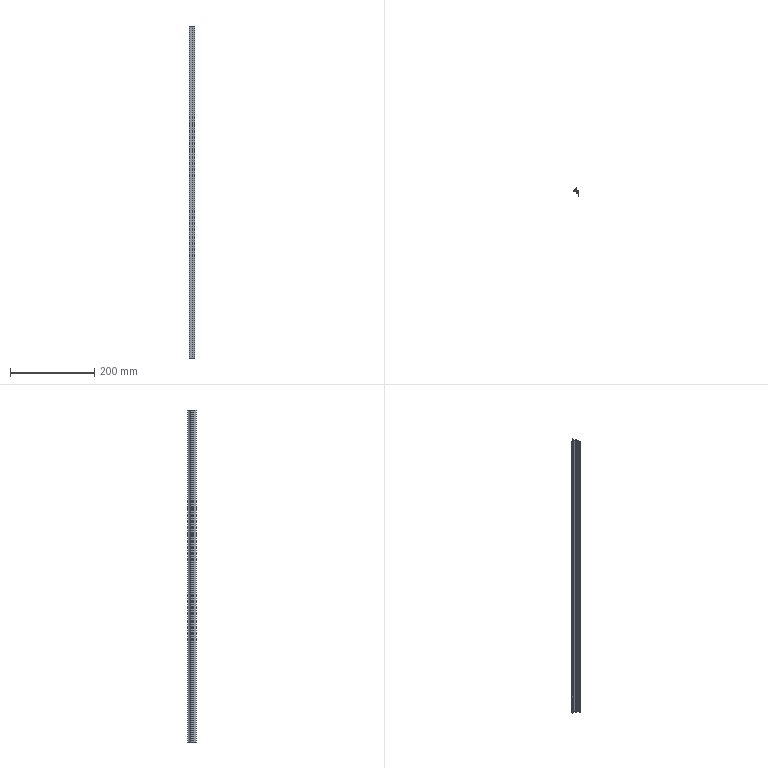Part | SolidWorks | features BaseBody 1, ICE 1, MoveFace 1 | 1 solid | 27 faces | box 14 x 20.3 x 786 mm | volume 40020 mm3 | plane 20 | cylinder 7 | commonest cylinder face diameters 0.387 x2 0.8 x2 0.4 x1 20 x1 22 x1
STEP:
#1=CARTESIAN_POINT('',(-5.304,-0.625,200.));
#2=VERTEX_POINT('',#1);
#3=CARTESIAN_POINT('',(-5.449,-0.8125,200.));
#4=VERTEX_POINT('',#3);
#5=CARTESIAN_POINT('',(-5.255,-0.8125,200.));
#6=DIRECTION('',(0.,0.,1.));
#7=DIRECTION('',(-1.,0.,0.));
#8=AXIS2_PLACEMENT_3D('',#5,#6,#7);
#9=CIRCLE('',#8,0.1937);
#10=EDGE_CURVE('',#2,#4,#9,.T.);
#11=ORIENTED_EDGE('',*,*,#10,.T.);
#12=CARTESIAN_POINT('',(-5.449,-0.8125,-586.));
#13=VERTEX_POINT('',#12);
#14=CARTESIAN_POINT('',(-5.449,-0.8125,230.));
#15=DIRECTION('',(0.,0.,-1.));
#16=VECTOR('',#15,1000.);
#17=LINE('',#14,#16);
#18=EDGE_CURVE('',#4,#13,#17,.T.);
#19=ORIENTED_EDGE('',*,*,#18,.T.);
#20=CARTESIAN_POINT('',(-5.304,-0.625,-586.));
#21=VERTEX_POINT('',#20);
#22=CARTESIAN_POINT('',(-5.255,-0.8125,-586.));
#23=DIRECTION('',(0.,0.,-1.));
#24=DIRECTION('',(1.,0.,0.));
#25=AXIS2_PLACEMENT_3D('',#22,#23,#24);
#26=CIRCLE('',#25,0.1937);
#27=EDGE_CURVE('',#13,#21,#26,.T.);
#28=ORIENTED_EDGE('',*,*,#27,.T.);
#29=CARTESIAN_POINT('',(-5.304,-0.625,230.));
#30=DIRECTION('',(0.,0.,-1.));
#31=VECTOR('',#30,1000.);
#32=LINE('',#29,#31);
#33=EDGE_CURVE('',#2,#21,#32,.T.);
#34=ORIENTED_EDGE('',*,*,#33,.F.);
#35=EDGE_LOOP('',(#11,#19,#28,#34));
#36=FACE_OUTER_BOUND('',#35,.T.);
#37=CARTESIAN_POINT('',(-5.255,-0.8125,230.));
#38=DIRECTION('',(0.,0.,-1.));
#39=DIRECTION('',(-1.,0.,0.));
#40=AXIS2_PLACEMENT_3D('',#37,#38,#39);
#41=CYLINDRICAL_SURFACE('',#40,0.1937);
#42=ADVANCED_FACE('',(#36),#41,.F.);
#43=CARTESIAN_POINT('',(5.,-1.,-586.));
#44=VERTEX_POINT('',#43);
#45=CARTESIAN_POINT('',(5.,-14.3,-586.));
#46=VERTEX_POINT('',#45);
#47=CARTESIAN_POINT('',(5.,29.623,-586.));
#48=DIRECTION('',(0.,-1.,0.));
#49=VECTOR('',#48,1000.);
#50=LINE('',#47,#49);
#51=EDGE_CURVE('',#44,#46,#50,.T.);
#52=ORIENTED_EDGE('',*,*,#51,.F.);
#53=CARTESIAN_POINT('',(5.,-1.,200.));
#54=VERTEX_POINT('',#53);
#55=CARTESIAN_POINT('',(5.,-1.,230.));
#56=DIRECTION('',(0.,0.,-1.));
#57=VECTOR('',#56,1000.);
#58=LINE('',#55,#57);
#59=EDGE_CURVE('',#54,#44,#58,.T.);
#60=ORIENTED_EDGE('',*,*,#59,.F.);
#61=CARTESIAN_POINT('',(5.,-14.3,200.));
#62=VERTEX_POINT('',#61);
#63=CARTESIAN_POINT('',(5.,-14.3,200.));
#64=DIRECTION('',(0.,1.,0.));
#65=VECTOR('',#64,1000.);
#66=LINE('',#63,#65);
#67=EDGE_CURVE('',#62,#54,#66,.T.);
#68=ORIENTED_EDGE('',*,*,#67,.F.);
#69=CARTESIAN_POINT('',(5.,-14.3,230.));
#70=DIRECTION('',(0.,0.,1.));
#71=VECTOR('',#70,1000.);
#72=LINE('',#69,#71);
#73=EDGE_CURVE('',#46,#62,#72,.T.);
#74=ORIENTED_EDGE('',*,*,#73,.F.);
#75=EDGE_LOOP('',(#52,#60,#68,#74));
#76=FACE_OUTER_BOUND('',#75,.T.);
#77=CARTESIAN_POINT('',(5.,-14.3,230.));
#78=DIRECTION('',(-1.,0.,0.));
#79=DIRECTION('',(0.,0.,1.));
#80=AXIS2_PLACEMENT_3D('',#77,#78,#79);
#81=PLANE('',#80);
#82=ADVANCED_FACE('',(#76),#81,.F.);
#83=CARTESIAN_POINT('',(-9.,-2.,-586.));
#84=VERTEX_POINT('',#83);
#85=CARTESIAN_POINT('',(-9.,-2.,200.));
#86=VERTEX_POINT('',#85);
#87=CARTESIAN_POINT('',(-9.,-2.,230.));
#88=DIRECTION('',(0.,0.,1.));
#89=VECTOR('',#88,1000.);
#90=LINE('',#87,#89);
#91=EDGE_CURVE('',#84,#86,#90,.T.);
#92=ORIENTED_EDGE('',*,*,#91,.F.);
#93=CARTESIAN_POINT('',(0.9,-2.,-586.));
#94=VERTEX_POINT('',#93);
#95=CARTESIAN_POINT('',(5.,-2.,-586.));
#96=DIRECTION('',(-1.,0.,0.));
#97=VECTOR('',#96,1000.);
#98=LINE('',#95,#97);
#99=EDGE_CURVE('',#94,#84,#98,.T.);
#100=ORIENTED_EDGE('',*,*,#99,.F.);
#101=CARTESIAN_POINT('',(0.9,-2.,200.));
#102=VERTEX_POINT('',#101);
#103=CARTESIAN_POINT('',(0.9,-2.,230.));
#104=DIRECTION('',(0.,0.,-1.));
#105=VECTOR('',#104,1000.);
#106=LINE('',#103,#105);
#107=EDGE_CURVE('',#102,#94,#106,.T.);
#108=ORIENTED_EDGE('',*,*,#107,.F.);
#109=CARTESIAN_POINT('',(5.,-2.,200.));
#110=DIRECTION('',(1.,0.,0.));
#111=VECTOR('',#110,1000.);
#112=LINE('',#109,#111);
#113=EDGE_CURVE('',#86,#102,#112,.T.);
#114=ORIENTED_EDGE('',*,*,#113,.F.);
#115=EDGE_LOOP('',(#92,#100,#108,#114));
#116=FACE_OUTER_BOUND('',#115,.T.);
#117=CARTESIAN_POINT('',(-9.,-2.,230.));
#118=DIRECTION('',(0.,1.,0.));
#119=DIRECTION('',(0.,0.,1.));
#120=AXIS2_PLACEMENT_3D('',#117,#118,#119);
#121=PLANE('',#120);
#122=ADVANCED_FACE('',(#116),#121,.F.);
#123=CARTESIAN_POINT('',(4.,-6.,200.));
#124=VERTEX_POINT('',#123);
#125=CARTESIAN_POINT('',(4.,-3.,200.));
#126=VERTEX_POINT('',#125);
#127=CARTESIAN_POINT('',(4.,29.623,200.));
#128=DIRECTION('',(0.,1.,0.));
#129=VECTOR('',#128,1000.);
#130=LINE('',#127,#129);
#131=EDGE_CURVE('',#124,#126,#130,.T.);
#132=ORIENTED_EDGE('',*,*,#131,.F.);
#133=CARTESIAN_POINT('',(1.,-6.,200.));
#134=VERTEX_POINT('',#133);
#135=CARTESIAN_POINT('',(5.,-6.,200.));
#136=DIRECTION('',(1.,0.,0.));
#137=VECTOR('',#136,1000.);
#138=LINE('',#135,#137);
#139=EDGE_CURVE('',#134,#124,#138,.T.);
#140=ORIENTED_EDGE('',*,*,#139,.F.);
#141=CARTESIAN_POINT('',(1.,-6.7,200.));
#142=VERTEX_POINT('',#141);
#143=CARTESIAN_POINT('',(1.,-6.,200.));
#144=DIRECTION('',(0.,-1.,0.));
#145=VECTOR('',#144,1000.);
#146=LINE('',#143,#145);
#147=EDGE_CURVE('',#134,#142,#146,.T.);
#148=ORIENTED_EDGE('',*,*,#147,.T.);
#149=CARTESIAN_POINT('',(-1.7,-6.7,200.));
#150=VERTEX_POINT('',#149);
#151=CARTESIAN_POINT('',(5.,-6.7,200.));
#152=DIRECTION('',(1.,0.,0.));
#153=VECTOR('',#152,1000.);
#154=LINE('',#151,#153);
#155=EDGE_CURVE('',#150,#142,#154,.T.);
#156=ORIENTED_EDGE('',*,*,#155,.F.);
#157=CARTESIAN_POINT('',(-1.7,-7.7,200.));
#158=VERTEX_POINT('',#157);
#159=CARTESIAN_POINT('',(-1.7,-6.7,200.));
#160=DIRECTION('',(0.,-1.,0.));
#161=VECTOR('',#160,1000.);
#162=LINE('',#159,#161);
#163=EDGE_CURVE('',#150,#158,#162,.T.);
#164=ORIENTED_EDGE('',*,*,#163,.T.);
#165=CARTESIAN_POINT('',(4.,-7.7,200.));
#166=VERTEX_POINT('',#165);
#167=CARTESIAN_POINT('',(5.,-7.7,200.));
#168=DIRECTION('',(-1.,0.,0.));
#169=VECTOR('',#168,1000.);
#170=LINE('',#167,#169);
#171=EDGE_CURVE('',#166,#158,#170,.T.);
#172=ORIENTED_EDGE('',*,*,#171,.F.);
#173=CARTESIAN_POINT('',(4.,-14.3,200.));
#174=VERTEX_POINT('',#173);
#175=CARTESIAN_POINT('',(4.,29.623,200.));
#176=DIRECTION('',(0.,1.,0.));
#177=VECTOR('',#176,1000.);
#178=LINE('',#175,#177);
#179=EDGE_CURVE('',#174,#166,#178,.T.);
#180=ORIENTED_EDGE('',*,*,#179,.F.);
#181=CARTESIAN_POINT('',(5.,-14.3,200.));
#182=DIRECTION('',(-1.,0.,0.));
#183=VECTOR('',#182,1000.);
#184=LINE('',#181,#183);
#185=EDGE_CURVE('',#62,#174,#184,.T.);
#186=ORIENTED_EDGE('',*,*,#185,.F.);
#187=ORIENTED_EDGE('',*,*,#67,.T.);
#188=CARTESIAN_POINT('',(-5.207,-1.,200.));
#189=VERTEX_POINT('',#188);
#190=CARTESIAN_POINT('',(5.,-1.,200.));
#191=DIRECTION('',(1.,0.,0.));
#192=VECTOR('',#191,1000.);
#193=LINE('',#190,#192);
#194=EDGE_CURVE('',#189,#54,#193,.T.);
#195=ORIENTED_EDGE('',*,*,#194,.F.);
#196=CARTESIAN_POINT('',(-5.255,-0.8125,200.));
#197=DIRECTION('',(0.,0.,1.));
#198=DIRECTION('',(-1.,0.,0.));
#199=AXIS2_PLACEMENT_3D('',#196,#197,#198);
#200=CIRCLE('',#199,0.1937);
#201=EDGE_CURVE('',#4,#189,#200,.T.);
#202=ORIENTED_EDGE('',*,*,#201,.F.);
#203=ORIENTED_EDGE('',*,*,#10,.F.);
#204=CARTESIAN_POINT('',(-1.368,3.063,200.));
#205=VERTEX_POINT('',#204);
#206=CARTESIAN_POINT('',(-10.628,9.,200.));
#207=DIRECTION('',(0.,0.,1.));
#208=DIRECTION('',(-1.,0.,0.));
#209=AXIS2_PLACEMENT_3D('',#206,#207,#208);
#210=CIRCLE('',#209,11.);
#211=EDGE_CURVE('',#2,#205,#210,.T.);
#212=ORIENTED_EDGE('',*,*,#211,.T.);
#213=CARTESIAN_POINT('',(-1.,2.955,200.));
#214=VERTEX_POINT('',#213);
#215=CARTESIAN_POINT('',(-1.2,2.955,200.));
#216=DIRECTION('',(0.,0.,1.));
#217=DIRECTION('',(-1.,0.,0.));
#218=AXIS2_PLACEMENT_3D('',#215,#216,#217);
#219=CIRCLE('',#218,0.2);
#220=EDGE_CURVE('',#214,#205,#219,.T.);
#221=ORIENTED_EDGE('',*,*,#220,.F.);
#222=CARTESIAN_POINT('',(-1.,1.5,200.));
#223=VERTEX_POINT('',#222);
#224=CARTESIAN_POINT('',(-1.,2.955,200.));
#225=DIRECTION('',(0.,1.,0.));
#226=VECTOR('',#225,1000.);
#227=LINE('',#224,#226);
#228=EDGE_CURVE('',#223,#214,#227,.T.);
#229=ORIENTED_EDGE('',*,*,#228,.F.);
#230=CARTESIAN_POINT('',(0.,1.5,200.));
#231=VERTEX_POINT('',#230);
#232=CARTESIAN_POINT('',(-1.,1.5,200.));
#233=DIRECTION('',(-1.,0.,0.));
#234=VECTOR('',#233,1000.);
#235=LINE('',#232,#234);
#236=EDGE_CURVE('',#231,#223,#235,.T.);
#237=ORIENTED_EDGE('',*,*,#236,.F.);
#238=CARTESIAN_POINT('',(0.,6.,200.));
#239=VERTEX_POINT('',#238);
#240=CARTESIAN_POINT('',(0.,1.5,200.));
#241=DIRECTION('',(0.,-1.,0.));
#242=VECTOR('',#241,1000.);
#243=LINE('',#240,#242);
#244=EDGE_CURVE('',#239,#231,#243,.T.);
#245=ORIENTED_EDGE('',*,*,#244,.F.);
#246=CARTESIAN_POINT('',(-0.8,6.,200.));
#247=VERTEX_POINT('',#246);
#248=CARTESIAN_POINT('',(0.,6.,200.));
#249=DIRECTION('',(1.,0.,0.));
#250=VECTOR('',#249,1000.);
#251=LINE('',#248,#250);
#252=EDGE_CURVE('',#247,#239,#251,.T.);
#253=ORIENTED_EDGE('',*,*,#252,.F.);
#254=CARTESIAN_POINT('',(-1.178,5.731,200.));
#255=VERTEX_POINT('',#254);
#256=CARTESIAN_POINT('',(-0.8,5.6,200.));
#257=DIRECTION('',(0.,0.,1.));
#258=DIRECTION('',(-1.,0.,0.));
#259=AXIS2_PLACEMENT_3D('',#256,#257,#258);
#260=CIRCLE('',#259,0.4);
#261=EDGE_CURVE('',#247,#255,#260,.T.);
#262=ORIENTED_EDGE('',*,*,#261,.T.);
#263=CARTESIAN_POINT('',(-8.678,-0.8077,200.));
#264=VERTEX_POINT('',#263);
#265=CARTESIAN_POINT('',(-10.628,9.,200.));
#266=DIRECTION('',(0.,0.,1.));
#267=DIRECTION('',(-1.,0.,0.));
#268=AXIS2_PLACEMENT_3D('',#265,#266,#267);
#269=CIRCLE('',#268,10.);
#270=EDGE_CURVE('',#264,#255,#269,.T.);
#271=ORIENTED_EDGE('',*,*,#270,.F.);
#272=CARTESIAN_POINT('',(-9.,-1.2,200.));
#273=VERTEX_POINT('',#272);
#274=CARTESIAN_POINT('',(-8.6,-1.2,200.));
#275=DIRECTION('',(0.,0.,1.));
#276=DIRECTION('',(-1.,0.,0.));
#277=AXIS2_PLACEMENT_3D('',#274,#275,#276);
#278=CIRCLE('',#277,0.4);
#279=EDGE_CURVE('',#264,#273,#278,.T.);
#280=ORIENTED_EDGE('',*,*,#279,.T.);
#281=CARTESIAN_POINT('',(-9.,8.,200.));
#282=DIRECTION('',(0.,-1.,0.));
#283=VECTOR('',#282,1000.);
#284=LINE('',#281,#283);
#285=EDGE_CURVE('',#273,#86,#284,.T.);
#286=ORIENTED_EDGE('',*,*,#285,.T.);
#287=ORIENTED_EDGE('',*,*,#113,.T.);
#288=CARTESIAN_POINT('',(0.9,-3.,200.));
#289=VERTEX_POINT('',#288);
#290=CARTESIAN_POINT('',(0.9,29.623,200.));
#291=DIRECTION('',(0.,1.,0.));
#292=VECTOR('',#291,1000.);
#293=LINE('',#290,#292);
#294=EDGE_CURVE('',#289,#102,#293,.T.);
#295=ORIENTED_EDGE('',*,*,#294,.F.);
#296=CARTESIAN_POINT('',(5.,-3.,200.));
#297=DIRECTION('',(-1.,0.,0.));
#298=VECTOR('',#297,1000.);
#299=LINE('',#296,#298);
#300=EDGE_CURVE('',#126,#289,#299,.T.);
#301=ORIENTED_EDGE('',*,*,#300,.F.);
#302=EDGE_LOOP('',(#132,#140,#148,#156,#164,#172,#180,#186,#187,#195,#202,#203,#212,#221,#229,#237,#245,#253,#262,#271,#280,#286,#287,#295,#301));
#303=FACE_OUTER_BOUND('',#302,.T.);
#304=CARTESIAN_POINT('',(5.,29.623,200.));
#305=DIRECTION('',(0.,0.,-1.));
#306=DIRECTION('',(-1.,0.,0.));
#307=AXIS2_PLACEMENT_3D('',#304,#305,#306);
#308=PLANE('',#307);
#309=ADVANCED_FACE('',(#303),#308,.F.);
#310=ORIENTED_EDGE('',*,*,#185,.T.);
#311=CARTESIAN_POINT('',(4.,-14.3,-586.));
#312=VERTEX_POINT('',#311);
#313=CARTESIAN_POINT('',(4.,-14.3,230.));
#314=DIRECTION('',(0.,0.,1.));
#315=VECTOR('',#314,1000.);
#316=LINE('',#313,#315);
#317=EDGE_CURVE('',#312,#174,#316,.T.);
#318=ORIENTED_EDGE('',*,*,#317,.F.);
#319=CARTESIAN_POINT('',(5.,-14.3,-586.));
#320=DIRECTION('',(-1.,0.,0.));
#321=VECTOR('',#320,1000.);
#322=LINE('',#319,#321);
#323=EDGE_CURVE('',#46,#312,#322,.T.);
#324=ORIENTED_EDGE('',*,*,#323,.F.);
#325=ORIENTED_EDGE('',*,*,#73,.T.);
#326=EDGE_LOOP('',(#310,#318,#324,#325));
#327=FACE_OUTER_BOUND('',#326,.T.);
#328=CARTESIAN_POINT('',(4.,-14.3,230.));
#329=DIRECTION('',(0.,1.,0.));
#330=DIRECTION('',(0.,0.,1.));
#331=AXIS2_PLACEMENT_3D('',#328,#329,#330);
#332=PLANE('',#331);
#333=ADVANCED_FACE('',(#327),#332,.F.);
#334=ORIENTED_EDGE('',*,*,#51,.T.);
#335=ORIENTED_EDGE('',*,*,#323,.T.);
#336=CARTESIAN_POINT('',(4.,-7.7,-586.));
#337=VERTEX_POINT('',#336);
#338=CARTESIAN_POINT('',(4.,-7.7,-586.));
#339=DIRECTION('',(0.,-1.,0.));
#340=VECTOR('',#339,1000.);
#341=LINE('',#338,#340);
#342=EDGE_CURVE('',#337,#312,#341,.T.);
#343=ORIENTED_EDGE('',*,*,#342,.F.);
#344=CARTESIAN_POINT('',(-1.7,-7.7,-586.));
#345=VERTEX_POINT('',#344);
#346=CARTESIAN_POINT('',(-1.7,-7.7,-586.));
#347=DIRECTION('',(1.,0.,0.));
#348=VECTOR('',#347,1000.);
#349=LINE('',#346,#348);
#350=EDGE_CURVE('',#345,#337,#349,.T.);
#351=ORIENTED_EDGE('',*,*,#350,.F.);
#352=CARTESIAN_POINT('',(-1.7,-6.7,-586.));
#353=VERTEX_POINT('',#352);
#354=CARTESIAN_POINT('',(-1.7,29.623,-586.));
#355=DIRECTION('',(0.,1.,0.));
#356=VECTOR('',#355,1000.);
#357=LINE('',#354,#356);
#358=EDGE_CURVE('',#345,#353,#357,.T.);
#359=ORIENTED_EDGE('',*,*,#358,.T.);
#360=CARTESIAN_POINT('',(1.,-6.7,-586.));
#361=VERTEX_POINT('',#360);
#362=CARTESIAN_POINT('',(1.,-6.7,-586.));
#363=DIRECTION('',(-1.,0.,0.));
#364=VECTOR('',#363,1000.);
#365=LINE('',#362,#364);
#366=EDGE_CURVE('',#361,#353,#365,.T.);
#367=ORIENTED_EDGE('',*,*,#366,.F.);
#368=CARTESIAN_POINT('',(1.,-6.,-586.));
#369=VERTEX_POINT('',#368);
#370=CARTESIAN_POINT('',(1.,29.623,-586.));
#371=DIRECTION('',(0.,1.,0.));
#372=VECTOR('',#371,1000.);
#373=LINE('',#370,#372);
#374=EDGE_CURVE('',#361,#369,#373,.T.);
#375=ORIENTED_EDGE('',*,*,#374,.T.);
#376=CARTESIAN_POINT('',(4.,-6.,-586.));
#377=VERTEX_POINT('',#376);
#378=CARTESIAN_POINT('',(4.,-6.,-586.));
#379=DIRECTION('',(-1.,0.,0.));
#380=VECTOR('',#379,1000.);
#381=LINE('',#378,#380);
#382=EDGE_CURVE('',#377,#369,#381,.T.);
#383=ORIENTED_EDGE('',*,*,#382,.F.);
#384=CARTESIAN_POINT('',(4.,-3.,-586.));
#385=VERTEX_POINT('',#384);
#386=CARTESIAN_POINT('',(4.,-3.,-586.));
#387=DIRECTION('',(0.,-1.,0.));
#388=VECTOR('',#387,1000.);
#389=LINE('',#386,#388);
#390=EDGE_CURVE('',#385,#377,#389,.T.);
#391=ORIENTED_EDGE('',*,*,#390,.F.);
#392=CARTESIAN_POINT('',(0.9,-3.,-586.));
#393=VERTEX_POINT('',#392);
#394=CARTESIAN_POINT('',(0.9,-3.,-586.));
#395=DIRECTION('',(1.,0.,0.));
#396=VECTOR('',#395,1000.);
#397=LINE('',#394,#396);
#398=EDGE_CURVE('',#393,#385,#397,.T.);
#399=ORIENTED_EDGE('',*,*,#398,.F.);
#400=CARTESIAN_POINT('',(0.9,-2.,-586.));
#401=DIRECTION('',(0.,-1.,0.));
#402=VECTOR('',#401,1000.);
#403=LINE('',#400,#402);
#404=EDGE_CURVE('',#94,#393,#403,.T.);
#405=ORIENTED_EDGE('',*,*,#404,.F.);
#406=ORIENTED_EDGE('',*,*,#99,.T.);
#407=CARTESIAN_POINT('',(-9.,-1.2,-586.));
#408=VERTEX_POINT('',#407);
#409=CARTESIAN_POINT('',(-9.,-1.2,-586.));
#410=DIRECTION('',(0.,-1.,0.));
#411=VECTOR('',#410,1000.);
#412=LINE('',#409,#411);
#413=EDGE_CURVE('',#408,#84,#412,.T.);
#414=ORIENTED_EDGE('',*,*,#413,.F.);
#415=CARTESIAN_POINT('',(-8.678,-0.8077,-586.));
#416=VERTEX_POINT('',#415);
#417=CARTESIAN_POINT('',(-8.6,-1.2,-586.));
#418=DIRECTION('',(0.,0.,-1.));
#419=DIRECTION('',(1.,0.,0.));
#420=AXIS2_PLACEMENT_3D('',#417,#418,#419);
#421=CIRCLE('',#420,0.4);
#422=EDGE_CURVE('',#408,#416,#421,.T.);
#423=ORIENTED_EDGE('',*,*,#422,.T.);
#424=CARTESIAN_POINT('',(-1.178,5.731,-586.));
#425=VERTEX_POINT('',#424);
#426=CARTESIAN_POINT('',(-10.628,9.,-586.));
#427=DIRECTION('',(0.,0.,-1.));
#428=DIRECTION('',(1.,0.,0.));
#429=AXIS2_PLACEMENT_3D('',#426,#427,#428);
#430=CIRCLE('',#429,10.);
#431=EDGE_CURVE('',#425,#416,#430,.T.);
#432=ORIENTED_EDGE('',*,*,#431,.F.);
#433=CARTESIAN_POINT('',(-0.8,6.,-586.));
#434=VERTEX_POINT('',#433);
#435=CARTESIAN_POINT('',(-0.8,5.6,-586.));
#436=DIRECTION('',(0.,0.,-1.));
#437=DIRECTION('',(1.,0.,0.));
#438=AXIS2_PLACEMENT_3D('',#435,#436,#437);
#439=CIRCLE('',#438,0.4);
#440=EDGE_CURVE('',#425,#434,#439,.T.);
#441=ORIENTED_EDGE('',*,*,#440,.T.);
#442=CARTESIAN_POINT('',(0.,6.,-586.));
#443=VERTEX_POINT('',#442);
#444=CARTESIAN_POINT('',(0.,6.,-586.));
#445=DIRECTION('',(-1.,0.,0.));
#446=VECTOR('',#445,1000.);
#447=LINE('',#444,#446);
#448=EDGE_CURVE('',#443,#434,#447,.T.);
#449=ORIENTED_EDGE('',*,*,#448,.F.);
#450=CARTESIAN_POINT('',(0.,1.5,-586.));
#451=VERTEX_POINT('',#450);
#452=CARTESIAN_POINT('',(0.,1.5,-586.));
#453=DIRECTION('',(0.,1.,0.));
#454=VECTOR('',#453,1000.);
#455=LINE('',#452,#454);
#456=EDGE_CURVE('',#451,#443,#455,.T.);
#457=ORIENTED_EDGE('',*,*,#456,.F.);
#458=CARTESIAN_POINT('',(-1.,1.5,-586.));
#459=VERTEX_POINT('',#458);
#460=CARTESIAN_POINT('',(-1.,1.5,-586.));
#461=DIRECTION('',(1.,0.,0.));
#462=VECTOR('',#461,1000.);
#463=LINE('',#460,#462);
#464=EDGE_CURVE('',#459,#451,#463,.T.);
#465=ORIENTED_EDGE('',*,*,#464,.F.);
#466=CARTESIAN_POINT('',(-1.,2.955,-586.));
#467=VERTEX_POINT('',#466);
#468=CARTESIAN_POINT('',(-1.,2.955,-586.));
#469=DIRECTION('',(0.,-1.,0.));
#470=VECTOR('',#469,1000.);
#471=LINE('',#468,#470);
#472=EDGE_CURVE('',#467,#459,#471,.T.);
#473=ORIENTED_EDGE('',*,*,#472,.F.);
#474=CARTESIAN_POINT('',(-1.368,3.063,-586.));
#475=VERTEX_POINT('',#474);
#476=CARTESIAN_POINT('',(-1.2,2.955,-586.));
#477=DIRECTION('',(0.,0.,-1.));
#478=DIRECTION('',(1.,0.,0.));
#479=AXIS2_PLACEMENT_3D('',#476,#477,#478);
#480=CIRCLE('',#479,0.2);
#481=EDGE_CURVE('',#475,#467,#480,.T.);
#482=ORIENTED_EDGE('',*,*,#481,.F.);
#483=CARTESIAN_POINT('',(-10.628,9.,-586.));
#484=DIRECTION('',(0.,0.,-1.));
#485=DIRECTION('',(1.,0.,0.));
#486=AXIS2_PLACEMENT_3D('',#483,#484,#485);
#487=CIRCLE('',#486,11.);
#488=EDGE_CURVE('',#475,#21,#487,.T.);
#489=ORIENTED_EDGE('',*,*,#488,.T.);
#490=ORIENTED_EDGE('',*,*,#27,.F.);
#491=CARTESIAN_POINT('',(-5.207,-1.,-586.));
#492=VERTEX_POINT('',#491);
#493=CARTESIAN_POINT('',(-5.255,-0.8125,-586.));
#494=DIRECTION('',(0.,0.,-1.));
#495=DIRECTION('',(1.,0.,0.));
#496=AXIS2_PLACEMENT_3D('',#493,#494,#495);
#497=CIRCLE('',#496,0.1937);
#498=EDGE_CURVE('',#492,#13,#497,.T.);
#499=ORIENTED_EDGE('',*,*,#498,.F.);
#500=CARTESIAN_POINT('',(5.,-1.,-586.));
#501=DIRECTION('',(-1.,0.,0.));
#502=VECTOR('',#501,1000.);
#503=LINE('',#500,#502);
#504=EDGE_CURVE('',#44,#492,#503,.T.);
#505=ORIENTED_EDGE('',*,*,#504,.F.);
#506=EDGE_LOOP('',(#334,#335,#343,#351,#359,#367,#375,#383,#391,#399,#405,#406,#414,#423,#432,#441,#449,#457,#465,#473,#482,#489,#490,#499,#505));
#507=FACE_OUTER_BOUND('',#506,.T.);
#508=CARTESIAN_POINT('',(5.,29.623,-586.));
#509=DIRECTION('',(0.,0.,1.));
#510=DIRECTION('',(1.,0.,0.));
#511=AXIS2_PLACEMENT_3D('',#508,#509,#510);
#512=PLANE('',#511);
#513=ADVANCED_FACE('',(#507),#512,.F.);
#514=ORIENTED_EDGE('',*,*,#59,.T.);
#515=ORIENTED_EDGE('',*,*,#504,.T.);
#516=CARTESIAN_POINT('',(-5.207,-1.,230.));
#517=DIRECTION('',(0.,0.,-1.));
#518=VECTOR('',#517,1000.);
#519=LINE('',#516,#518);
#520=EDGE_CURVE('',#189,#492,#519,.T.);
#521=ORIENTED_EDGE('',*,*,#520,.F.);
#522=ORIENTED_EDGE('',*,*,#194,.T.);
#523=EDGE_LOOP('',(#514,#515,#521,#522));
#524=FACE_OUTER_BOUND('',#523,.T.);
#525=CARTESIAN_POINT('',(5.,-1.,230.));
#526=DIRECTION('',(0.,-1.,0.));
#527=DIRECTION('',(0.,0.,-1.));
#528=AXIS2_PLACEMENT_3D('',#525,#526,#527);
#529=PLANE('',#528);
#530=ADVANCED_FACE('',(#524),#529,.F.);
#531=CARTESIAN_POINT('',(-9.,-1.2,230.));
#532=DIRECTION('',(0.,0.,1.));
#533=VECTOR('',#532,1000.);
#534=LINE('',#531,#533);
#535=EDGE_CURVE('',#408,#273,#534,.T.);
#536=ORIENTED_EDGE('',*,*,#535,.F.);
#537=ORIENTED_EDGE('',*,*,#413,.T.);
#538=ORIENTED_EDGE('',*,*,#91,.T.);
#539=ORIENTED_EDGE('',*,*,#285,.F.);
#540=EDGE_LOOP('',(#536,#537,#538,#539));
#541=FACE_OUTER_BOUND('',#540,.T.);
#542=CARTESIAN_POINT('',(-9.,-1.2,230.));
#543=DIRECTION('',(1.,0.,0.));
#544=DIRECTION('',(0.,0.,-1.));
#545=AXIS2_PLACEMENT_3D('',#542,#543,#544);
#546=PLANE('',#545);
#547=ADVANCED_FACE('',(#541),#546,.F.);
#548=ORIENTED_EDGE('',*,*,#294,.T.);
#549=ORIENTED_EDGE('',*,*,#107,.T.);
#550=ORIENTED_EDGE('',*,*,#404,.T.);
#551=CARTESIAN_POINT('',(0.9,-3.,230.));
#552=DIRECTION('',(0.,0.,-1.));
#553=VECTOR('',#552,1000.);
#554=LINE('',#551,#553);
#555=EDGE_CURVE('',#289,#393,#554,.T.);
#556=ORIENTED_EDGE('',*,*,#555,.F.);
#557=EDGE_LOOP('',(#548,#549,#550,#556));
#558=FACE_OUTER_BOUND('',#557,.T.);
#559=CARTESIAN_POINT('',(0.9,-2.,230.));
#560=DIRECTION('',(1.,0.,0.));
#561=DIRECTION('',(0.,0.,-1.));
#562=AXIS2_PLACEMENT_3D('',#559,#560,#561);
#563=PLANE('',#562);
#564=ADVANCED_FACE('',(#558),#563,.F.);
#565=ORIENTED_EDGE('',*,*,#300,.T.);
#566=ORIENTED_EDGE('',*,*,#555,.T.);
#567=ORIENTED_EDGE('',*,*,#398,.T.);
#568=CARTESIAN_POINT('',(4.,-3.,230.));
#569=DIRECTION('',(0.,0.,-1.));
#570=VECTOR('',#569,1000.);
#571=LINE('',#568,#570);
#572=EDGE_CURVE('',#126,#385,#571,.T.);
#573=ORIENTED_EDGE('',*,*,#572,.F.);
#574=EDGE_LOOP('',(#565,#566,#567,#573));
#575=FACE_OUTER_BOUND('',#574,.T.);
#576=CARTESIAN_POINT('',(0.9,-3.,230.));
#577=DIRECTION('',(0.,1.,0.));
#578=DIRECTION('',(0.,0.,1.));
#579=AXIS2_PLACEMENT_3D('',#576,#577,#578);
#580=PLANE('',#579);
#581=ADVANCED_FACE('',(#575),#580,.F.);
#582=ORIENTED_EDGE('',*,*,#131,.T.);
#583=ORIENTED_EDGE('',*,*,#572,.T.);
#584=ORIENTED_EDGE('',*,*,#390,.T.);
#585=CARTESIAN_POINT('',(4.,-6.,230.));
#586=DIRECTION('',(0.,0.,-1.));
#587=VECTOR('',#586,1000.);
#588=LINE('',#585,#587);
#589=EDGE_CURVE('',#124,#377,#588,.T.);
#590=ORIENTED_EDGE('',*,*,#589,.F.);
#591=EDGE_LOOP('',(#582,#583,#584,#590));
#592=FACE_OUTER_BOUND('',#591,.T.);
#593=CARTESIAN_POINT('',(4.,-3.,230.));
#594=DIRECTION('',(1.,0.,0.));
#595=DIRECTION('',(0.,0.,-1.));
#596=AXIS2_PLACEMENT_3D('',#593,#594,#595);
#597=PLANE('',#596);
#598=ADVANCED_FACE('',(#592),#597,.F.);
#599=ORIENTED_EDGE('',*,*,#139,.T.);
#600=ORIENTED_EDGE('',*,*,#589,.T.);
#601=ORIENTED_EDGE('',*,*,#382,.T.);
#602=CARTESIAN_POINT('',(1.,-6.,230.));
#603=DIRECTION('',(0.,0.,-1.));
#604=VECTOR('',#603,1000.);
#605=LINE('',#602,#604);
#606=EDGE_CURVE('',#134,#369,#605,.T.);
#607=ORIENTED_EDGE('',*,*,#606,.F.);
#608=EDGE_LOOP('',(#599,#600,#601,#607));
#609=FACE_OUTER_BOUND('',#608,.T.);
#610=CARTESIAN_POINT('',(4.,-6.,230.));
#611=DIRECTION('',(0.,-1.,0.));
#612=DIRECTION('',(0.,0.,-1.));
#613=AXIS2_PLACEMENT_3D('',#610,#611,#612);
#614=PLANE('',#613);
#615=ADVANCED_FACE('',(#609),#614,.F.);
#616=ORIENTED_EDGE('',*,*,#155,.T.);
#617=CARTESIAN_POINT('',(1.,-6.7,230.));
#618=DIRECTION('',(0.,0.,1.));
#619=VECTOR('',#618,1000.);
#620=LINE('',#617,#619);
#621=EDGE_CURVE('',#361,#142,#620,.T.);
#622=ORIENTED_EDGE('',*,*,#621,.F.);
#623=ORIENTED_EDGE('',*,*,#366,.T.);
#624=CARTESIAN_POINT('',(-1.7,-6.7,230.));
#625=DIRECTION('',(0.,0.,-1.));
#626=VECTOR('',#625,1000.);
#627=LINE('',#624,#626);
#628=EDGE_CURVE('',#150,#353,#627,.T.);
#629=ORIENTED_EDGE('',*,*,#628,.F.);
#630=EDGE_LOOP('',(#616,#622,#623,#629));
#631=FACE_OUTER_BOUND('',#630,.T.);
#632=CARTESIAN_POINT('',(1.,-6.7,230.));
#633=DIRECTION('',(0.,-1.,0.));
#634=DIRECTION('',(0.,0.,-1.));
#635=AXIS2_PLACEMENT_3D('',#632,#633,#634);
#636=PLANE('',#635);
#637=ADVANCED_FACE('',(#631),#636,.F.);
#638=ORIENTED_EDGE('',*,*,#171,.T.);
#639=CARTESIAN_POINT('',(-1.7,-7.7,230.));
#640=DIRECTION('',(0.,0.,1.));
#641=VECTOR('',#640,1000.);
#642=LINE('',#639,#641);
#643=EDGE_CURVE('',#345,#158,#642,.T.);
#644=ORIENTED_EDGE('',*,*,#643,.F.);
#645=ORIENTED_EDGE('',*,*,#350,.T.);
#646=CARTESIAN_POINT('',(4.,-7.7,230.));
#647=DIRECTION('',(0.,0.,-1.));
#648=VECTOR('',#647,1000.);
#649=LINE('',#646,#648);
#650=EDGE_CURVE('',#166,#337,#649,.T.);
#651=ORIENTED_EDGE('',*,*,#650,.F.);
#652=EDGE_LOOP('',(#638,#644,#645,#651));
#653=FACE_OUTER_BOUND('',#652,.T.);
#654=CARTESIAN_POINT('',(-1.7,-7.7,230.));
#655=DIRECTION('',(0.,1.,0.));
#656=DIRECTION('',(0.,0.,1.));
#657=AXIS2_PLACEMENT_3D('',#654,#655,#656);
#658=PLANE('',#657);
#659=ADVANCED_FACE('',(#653),#658,.F.);
#660=ORIENTED_EDGE('',*,*,#179,.T.);
#661=ORIENTED_EDGE('',*,*,#650,.T.);
#662=ORIENTED_EDGE('',*,*,#342,.T.);
#663=ORIENTED_EDGE('',*,*,#317,.T.);
#664=EDGE_LOOP('',(#660,#661,#662,#663));
#665=FACE_OUTER_BOUND('',#664,.T.);
#666=CARTESIAN_POINT('',(4.,-7.7,230.));
#667=DIRECTION('',(1.,0.,0.));
#668=DIRECTION('',(0.,0.,-1.));
#669=AXIS2_PLACEMENT_3D('',#666,#667,#668);
#670=PLANE('',#669);
#671=ADVANCED_FACE('',(#665),#670,.F.);
#672=ORIENTED_EDGE('',*,*,#18,.F.);
#673=ORIENTED_EDGE('',*,*,#201,.T.);
#674=ORIENTED_EDGE('',*,*,#520,.T.);
#675=ORIENTED_EDGE('',*,*,#498,.T.);
#676=EDGE_LOOP('',(#672,#673,#674,#675));
#677=FACE_OUTER_BOUND('',#676,.T.);
#678=CARTESIAN_POINT('',(-5.255,-0.8125,230.));
#679=DIRECTION('',(0.,0.,-1.));
#680=DIRECTION('',(-1.,0.,0.));
#681=AXIS2_PLACEMENT_3D('',#678,#679,#680);
#682=CYLINDRICAL_SURFACE('',#681,0.1937);
#683=ADVANCED_FACE('',(#677),#682,.F.);
#684=CARTESIAN_POINT('',(-1.,2.955,230.));
#685=DIRECTION('',(0.,0.,1.));
#686=VECTOR('',#685,1000.);
#687=LINE('',#684,#686);
#688=EDGE_CURVE('',#467,#214,#687,.T.);
#689=ORIENTED_EDGE('',*,*,#688,.F.);
#690=ORIENTED_EDGE('',*,*,#472,.T.);
#691=CARTESIAN_POINT('',(-1.,1.5,230.));
#692=DIRECTION('',(0.,0.,-1.));
#693=VECTOR('',#692,1000.);
#694=LINE('',#691,#693);
#695=EDGE_CURVE('',#223,#459,#694,.T.);
#696=ORIENTED_EDGE('',*,*,#695,.F.);
#697=ORIENTED_EDGE('',*,*,#228,.T.);
#698=EDGE_LOOP('',(#689,#690,#696,#697));
#699=FACE_OUTER_BOUND('',#698,.T.);
#700=CARTESIAN_POINT('',(-1.,2.955,230.));
#701=DIRECTION('',(1.,0.,0.));
#702=DIRECTION('',(0.,0.,-1.));
#703=AXIS2_PLACEMENT_3D('',#700,#701,#702);
#704=PLANE('',#703);
#705=ADVANCED_FACE('',(#699),#704,.F.);
#706=ORIENTED_EDGE('',*,*,#488,.F.);
#707=CARTESIAN_POINT('',(-1.368,3.063,230.));
#708=DIRECTION('',(0.,0.,1.));
#709=VECTOR('',#708,1000.);
#710=LINE('',#707,#709);
#711=EDGE_CURVE('',#475,#205,#710,.T.);
#712=ORIENTED_EDGE('',*,*,#711,.T.);
#713=ORIENTED_EDGE('',*,*,#211,.F.);
#714=ORIENTED_EDGE('',*,*,#33,.T.);
#715=EDGE_LOOP('',(#706,#712,#713,#714));
#716=FACE_OUTER_BOUND('',#715,.T.);
#717=CARTESIAN_POINT('',(-10.628,9.,230.));
#718=DIRECTION('',(0.,0.,-1.));
#719=DIRECTION('',(-1.,0.,0.));
#720=AXIS2_PLACEMENT_3D('',#717,#718,#719);
#721=CYLINDRICAL_SURFACE('',#720,11.);
#722=ADVANCED_FACE('',(#716),#721,.T.);
#723=CARTESIAN_POINT('',(-1.178,5.731,230.));
#724=DIRECTION('',(0.,0.,1.));
#725=VECTOR('',#724,1000.);
#726=LINE('',#723,#725);
#727=EDGE_CURVE('',#425,#255,#726,.T.);
#728=ORIENTED_EDGE('',*,*,#727,.F.);
#729=ORIENTED_EDGE('',*,*,#431,.T.);
#730=CARTESIAN_POINT('',(-8.678,-0.8077,230.));
#731=DIRECTION('',(0.,0.,-1.));
#732=VECTOR('',#731,1000.);
#733=LINE('',#730,#732);
#734=EDGE_CURVE('',#264,#416,#733,.T.);
#735=ORIENTED_EDGE('',*,*,#734,.F.);
#736=ORIENTED_EDGE('',*,*,#270,.T.);
#737=EDGE_LOOP('',(#728,#729,#735,#736));
#738=FACE_OUTER_BOUND('',#737,.T.);
#739=CARTESIAN_POINT('',(-10.628,9.,230.));
#740=DIRECTION('',(0.,0.,-1.));
#741=DIRECTION('',(-1.,0.,0.));
#742=AXIS2_PLACEMENT_3D('',#739,#740,#741);
#743=CYLINDRICAL_SURFACE('',#742,10.);
#744=ADVANCED_FACE('',(#738),#743,.F.);
#745=CARTESIAN_POINT('',(0.,1.5,230.));
#746=DIRECTION('',(0.,0.,1.));
#747=VECTOR('',#746,1000.);
#748=LINE('',#745,#747);
#749=EDGE_CURVE('',#451,#231,#748,.T.);
#750=ORIENTED_EDGE('',*,*,#749,.F.);
#751=ORIENTED_EDGE('',*,*,#456,.T.);
#752=CARTESIAN_POINT('',(0.,6.,230.));
#753=DIRECTION('',(0.,0.,-1.));
#754=VECTOR('',#753,1000.);
#755=LINE('',#752,#754);
#756=EDGE_CURVE('',#239,#443,#755,.T.);
#757=ORIENTED_EDGE('',*,*,#756,.F.);
#758=ORIENTED_EDGE('',*,*,#244,.T.);
#759=EDGE_LOOP('',(#750,#751,#757,#758));
#760=FACE_OUTER_BOUND('',#759,.T.);
#761=CARTESIAN_POINT('',(0.,1.5,230.));
#762=DIRECTION('',(-1.,0.,0.));
#763=DIRECTION('',(0.,0.,1.));
#764=AXIS2_PLACEMENT_3D('',#761,#762,#763);
#765=PLANE('',#764);
#766=ADVANCED_FACE('',(#760),#765,.F.);
#767=ORIENTED_EDGE('',*,*,#422,.F.);
#768=ORIENTED_EDGE('',*,*,#535,.T.);
#769=ORIENTED_EDGE('',*,*,#279,.F.);
#770=ORIENTED_EDGE('',*,*,#734,.T.);
#771=EDGE_LOOP('',(#767,#768,#769,#770));
#772=FACE_OUTER_BOUND('',#771,.T.);
#773=CARTESIAN_POINT('',(-8.6,-1.2,230.));
#774=DIRECTION('',(0.,0.,-1.));
#775=DIRECTION('',(-1.,0.,0.));
#776=AXIS2_PLACEMENT_3D('',#773,#774,#775);
#777=CYLINDRICAL_SURFACE('',#776,0.4);
#778=ADVANCED_FACE('',(#772),#777,.T.);
#779=ORIENTED_EDGE('',*,*,#147,.F.);
#780=ORIENTED_EDGE('',*,*,#606,.T.);
#781=ORIENTED_EDGE('',*,*,#374,.F.);
#782=ORIENTED_EDGE('',*,*,#621,.T.);
#783=EDGE_LOOP('',(#779,#780,#781,#782));
#784=FACE_OUTER_BOUND('',#783,.T.);
#785=CARTESIAN_POINT('',(1.,-6.,230.));
#786=DIRECTION('',(1.,0.,0.));
#787=DIRECTION('',(0.,0.,-1.));
#788=AXIS2_PLACEMENT_3D('',#785,#786,#787);
#789=PLANE('',#788);
#790=ADVANCED_FACE('',(#784),#789,.F.);
#791=ORIENTED_EDGE('',*,*,#163,.F.);
#792=ORIENTED_EDGE('',*,*,#628,.T.);
#793=ORIENTED_EDGE('',*,*,#358,.F.);
#794=ORIENTED_EDGE('',*,*,#643,.T.);
#795=EDGE_LOOP('',(#791,#792,#793,#794));
#796=FACE_OUTER_BOUND('',#795,.T.);
#797=CARTESIAN_POINT('',(-1.7,-6.7,230.));
#798=DIRECTION('',(1.,0.,0.));
#799=DIRECTION('',(0.,0.,-1.));
#800=AXIS2_PLACEMENT_3D('',#797,#798,#799);
#801=PLANE('',#800);
#802=ADVANCED_FACE('',(#796),#801,.F.);
#803=ORIENTED_EDGE('',*,*,#711,.F.);
#804=ORIENTED_EDGE('',*,*,#481,.T.);
#805=ORIENTED_EDGE('',*,*,#688,.T.);
#806=ORIENTED_EDGE('',*,*,#220,.T.);
#807=EDGE_LOOP('',(#803,#804,#805,#806));
#808=FACE_OUTER_BOUND('',#807,.T.);
#809=CARTESIAN_POINT('',(-1.2,2.955,230.));
#810=DIRECTION('',(0.,0.,-1.));
#811=DIRECTION('',(-1.,0.,0.));
#812=AXIS2_PLACEMENT_3D('',#809,#810,#811);
#813=CYLINDRICAL_SURFACE('',#812,0.2);
#814=ADVANCED_FACE('',(#808),#813,.F.);
#815=ORIENTED_EDGE('',*,*,#695,.T.);
#816=ORIENTED_EDGE('',*,*,#464,.T.);
#817=ORIENTED_EDGE('',*,*,#749,.T.);
#818=ORIENTED_EDGE('',*,*,#236,.T.);
#819=EDGE_LOOP('',(#815,#816,#817,#818));
#820=FACE_OUTER_BOUND('',#819,.T.);
#821=CARTESIAN_POINT('',(-1.,1.5,230.));
#822=DIRECTION('',(0.,1.,0.));
#823=DIRECTION('',(0.,0.,1.));
#824=AXIS2_PLACEMENT_3D('',#821,#822,#823);
#825=PLANE('',#824);
#826=ADVANCED_FACE('',(#820),#825,.F.);
#827=ORIENTED_EDGE('',*,*,#440,.F.);
#828=ORIENTED_EDGE('',*,*,#727,.T.);
#829=ORIENTED_EDGE('',*,*,#261,.F.);
#830=CARTESIAN_POINT('',(-0.8,6.,230.));
#831=DIRECTION('',(0.,0.,-1.));
#832=VECTOR('',#831,1000.);
#833=LINE('',#830,#832);
#834=EDGE_CURVE('',#247,#434,#833,.T.);
#835=ORIENTED_EDGE('',*,*,#834,.T.);
#836=EDGE_LOOP('',(#827,#828,#829,#835));
#837=FACE_OUTER_BOUND('',#836,.T.);
#838=CARTESIAN_POINT('',(-0.8,5.6,230.));
#839=DIRECTION('',(0.,0.,-1.));
#840=DIRECTION('',(-1.,0.,0.));
#841=AXIS2_PLACEMENT_3D('',#838,#839,#840);
#842=CYLINDRICAL_SURFACE('',#841,0.4);
#843=ADVANCED_FACE('',(#837),#842,.T.);
#844=ORIENTED_EDGE('',*,*,#756,.T.);
#845=ORIENTED_EDGE('',*,*,#448,.T.);
#846=ORIENTED_EDGE('',*,*,#834,.F.);
#847=ORIENTED_EDGE('',*,*,#252,.T.);
#848=EDGE_LOOP('',(#844,#845,#846,#847));
#849=FACE_OUTER_BOUND('',#848,.T.);
#850=CARTESIAN_POINT('',(0.,6.,230.));
#851=DIRECTION('',(0.,-1.,0.));
#852=DIRECTION('',(0.,0.,-1.));
#853=AXIS2_PLACEMENT_3D('',#850,#851,#852);
#854=PLANE('',#853);
#855=ADVANCED_FACE('',(#849),#854,.F.);
#856=CLOSED_SHELL('',(#42,#82,#122,#309,#333,#513,#530,#547,#564,#581,#598,#615,#637,#659,#671,#683,#705,#722,#744,#766,#778,#790,#802,#814,#826,#843,#855));
#857=MANIFOLD_SOLID_BREP('',#856);
#858=CARTESIAN_POINT('',(0.,0.,0.));
#859=DIRECTION('',(0.,0.,1.));
#860=DIRECTION('',(1.,0.,0.));
#861=AXIS2_PLACEMENT_3D('',#858,#859,#860);
#862=(LENGTH_UNIT()NAMED_UNIT(*)SI_UNIT(.MILLI.,.METRE.));
#863=UNCERTAINTY_MEASURE_WITH_UNIT(LENGTH_MEASURE(0.00001),#862,'','');
#864=(NAMED_UNIT(*)PLANE_ANGLE_UNIT()SI_UNIT($,.RADIAN.));
#865=(NAMED_UNIT(*)SI_UNIT($,.STERADIAN.)SOLID_ANGLE_UNIT());
#866=(GEOMETRIC_REPRESENTATION_CONTEXT(3)GLOBAL_UNCERTAINTY_ASSIGNED_CONTEXT((#863))GLOBAL_UNIT_ASSIGNED_CONTEXT((#862,#864,#865))REPRESENTATION_CONTEXT('',''));
#867=ADVANCED_BREP_SHAPE_REPRESENTATION('',(#857,#861),#866);